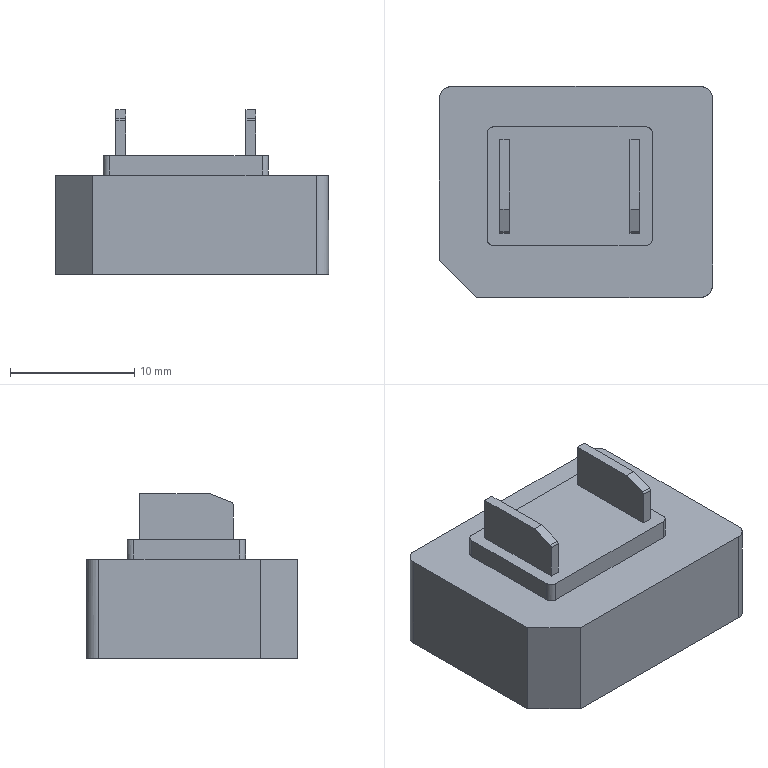NC program | PowerMill | posted by the shop | part box 22 x 17 x 13.286 mm
Lines 2696 to 5761 of 53717, first 2486 of 3066 lines:
( TOOL ID   D4C_1_1 )
( TOOL DIA. 4. TIP RAD 0 LENGTH 60.44 )
( Z = -5.38 )
T2 M6
T3
G91 G28 Z0
G0 G90 G54
M08
S18000 M3
X0 Y0 M8
G43 Z9.805 H2
X3.3 Y-4.574
Z.812
G1 Z-.388 F3600
X3.393 Y-4.374 F6000
X3.66 Y-3.797
X3.365 Y-3.66
X3.172 Y-3.54
X2.782 Y-3.172
X2.684 Y-3.041
X2.491 Y-2.684
X2.351 Y-2.196
X2.324 Y-1.708
Y.732
X.436 Y.731
G2 X-.364 Y-.069 I-.8 J0
G1 X-.636
G2 X-1.436 Y.731 I0 J.8
G1 Y1.674
G2 X-.636 Y2.473 I.8 J0
G1 X-.364
G2 X.436 Y1.674 I0 J-.8
G1 Y.731
X2.324 Y.732
Y4.148
X2.366 Y4.637
X2.534 Y5.125
X2.684 Y5.38
X2.873 Y5.613
X3.172 Y5.874
X3.585 Y6.101
X4.148 Y6.239
X5.125 Y6.249
X5.613 Y6.195
X5.907 Y6.101
X6.101 Y6.01
X6.589 Y5.645
X6.959 Y5.125
X7.077 Y4.829
X7.126 Y4.637
X7.168 Y4.148
Y-1.708
X7.142 Y-2.196
X7.077 Y-2.481
X7.002 Y-2.684
X6.707 Y-3.172
X6.589 Y-3.309
X6.127 Y-3.66
X5.613 Y-3.863
X5.125 Y-3.917
X4.148 Y-3.908
X3.66 Y-3.797
X3.393 Y-4.374
X-3.504 Y-4.099
X-3.657 Y-3.941
X-4.103 Y-3.479
X-4.148 Y-3.523
X-4.365 Y-3.66
X-4.637 Y-3.789
X-5.125 Y-3.905
X-6.101 Y-3.917
X-6.589 Y-3.869
X-7.077 Y-3.69
X-7.565 Y-3.333
X-7.709 Y-3.172
X-8.002 Y-2.684
X-8.142 Y-2.196
X-8.168 Y-1.708
Y4.148
X-8.126 Y4.637
X-8.053 Y4.901
X-7.959 Y5.125
X-7.62 Y5.613
X-7.077 Y6.023
X-6.908 Y6.101
X-6.589 Y6.2
X-6.101 Y6.249
X-5.125 Y6.237
X-4.637 Y6.121
X-4.148 Y5.857
X-3.873 Y5.613
X-3.66 Y5.345
X-3.534 Y5.125
X-3.366 Y4.637
X-3.324 Y4.148
Y-1.708
X-3.351 Y-2.196
X-3.49 Y-2.684
X-3.66 Y-3.005
X-3.786 Y-3.172
X-4.103 Y-3.479
X-3.657 Y-3.941
X2.918 Y-4.872 Z-.581
X3.035 Y-4.686
X3.373 Y-4.148
X3.172 Y-4.022
X2.789 Y-3.66
X2.684 Y-3.523
X2.493 Y-3.172
X2.351 Y-2.684
X2.324 Y-2.196
Y.972
X.436 Y.971
Y.268
G2 X-.367 Y-.532 I-.8 J0
G1 X-.639 Y-.531
G2 X-1.436 Y.269 I.003 J.8
G1 Y1.673
G2 X-.636 Y2.473 I.8 J0
G1 X-.364
G2 X.436 Y1.674 I0 J-.8
G1 Y.971
X2.324 Y.972
Y4.148
X2.366 Y4.637
X2.534 Y5.125
X2.684 Y5.38
X2.873 Y5.613
X3.172 Y5.874
X3.585 Y6.101
X4.148 Y6.239
X5.125 Y6.249
X5.613 Y6.195
X5.907 Y6.101
X6.101 Y6.01
X6.589 Y5.645
X6.959 Y5.125
X7.077 Y4.829
X7.127 Y4.637
X7.168 Y4.148
Y-2.196
X7.14 Y-2.684
X7.077 Y-2.963
X7. Y-3.172
X6.702 Y-3.66
X6.589 Y-3.791
X6.117 Y-4.148
X5.613 Y-4.345
X5.125 Y-4.4
X4.148 Y-4.39
X3.66 Y-4.28
X3.373 Y-4.148
X3.035 Y-4.686
G0 Z3.619
G1 X-8.196 Y-4.385 F10000
G0 Z.619
G1 Z-.581 F3600
X-8.033 Y-4.238 F6000
X-7.565 Y-3.815
X-7.704 Y-3.66
X-8. Y-3.172
X-8.141 Y-2.684
X-8.168 Y-2.196
Y4.148
X-8.126 Y4.637
X-8.053 Y4.901
X-7.959 Y5.125
X-7.62 Y5.613
X-7.077 Y6.023
X-6.908 Y6.101
X-6.589 Y6.2
X-6.101 Y6.249
X-5.125 Y6.237
X-4.637 Y6.121
X-4.148 Y5.857
X-3.873 Y5.613
X-3.66 Y5.345
X-3.534 Y5.125
X-3.366 Y4.637
X-3.324 Y4.148
Y-2.196
X-3.352 Y-2.684
X-3.493 Y-3.172
X-3.66 Y-3.487
X-3.79 Y-3.66
X-4.148 Y-4.005
X-4.374 Y-4.148
X-4.637 Y-4.271
X-5.125 Y-4.388
X-6.101 Y-4.4
X-6.589 Y-4.351
X-7.077 Y-4.172
X-7.565 Y-3.815
X-8.033 Y-4.238
G0 Z3.426
G1 X4.75 Y-5.738 F10000
G0 Z.426
G1 Z-.774 F3600
X4.752 Y-5.518 F6000
X4.759 Y-4.878
X4.148 Y-4.873
X3.66 Y-4.762
X3.385 Y-4.637
X3.172 Y-4.505
X2.795 Y-4.148
X2.684 Y-4.005
X2.496 Y-3.66
X2.352 Y-3.172
X2.324 Y-2.684
Y.725
X.436 Y.724
X.437 Y-.225
G2 X-.367 Y-1.025 I-.8 J0
G1 X-.639 Y-1.024
G2 X-1.436 Y-.224 I.004 J.8
G1 Y1.673
G2 X-.636 Y2.473 I.8 J0
G1 X-.364
G2 X.436 Y1.674 I0 J-.8
G1 Y.724
X2.324 Y.725
Y4.148
X2.366 Y4.637
X2.534 Y5.125
X2.684 Y5.38
X2.873 Y5.613
X3.172 Y5.874
X3.585 Y6.101
X4.148 Y6.239
X5.125 Y6.249
X5.613 Y6.195
X5.907 Y6.101
X6.101 Y6.01
X6.589 Y5.645
X6.959 Y5.125
X7.077 Y4.829
X7.127 Y4.637
X7.168 Y4.148
Y-2.684
X7.14 Y-3.172
X7.077 Y-3.445
X6.998 Y-3.66
X6.698 Y-4.148
X6.589 Y-4.273
X6.106 Y-4.637
X5.613 Y-4.828
X5.125 Y-4.882
X4.759 Y-4.878
X4.752 Y-5.518
X-2.974 Y-4.488
X-3.149 Y-4.355
X-3.66 Y-3.97
X-3.795 Y-4.148
X-4.148 Y-4.487
X-4.386 Y-4.637
X-4.637 Y-4.753
X-5.125 Y-4.87
X-6.101 Y-4.882
X-6.589 Y-4.833
X-7.077 Y-4.654
X-7.565 Y-4.297
X-7.698 Y-4.148
X-7.998 Y-3.66
X-8.14 Y-3.172
X-8.168 Y-2.684
Y4.148
X-8.126 Y4.637
X-8.053 Y4.901
X-7.959 Y5.125
X-7.62 Y5.613
X-7.077 Y6.023
X-6.908 Y6.101
X-6.589 Y6.2
X-6.101 Y6.249
X-5.125 Y6.237
X-4.637 Y6.121
X-4.148 Y5.857
X-3.873 Y5.613
X-3.66 Y5.345
X-3.534 Y5.125
X-3.366 Y4.637
X-3.324 Y4.148
Y-.092
Y-2.196
Y-2.198
Y-2.2
Y-2.684
X-3.352 Y-3.172
X-3.495 Y-3.66
X-3.66 Y-3.97
X-3.149 Y-4.355
G0 Z3.233
G1 X7.163 Y-5.334 F10000
G0 Z.233
G1 Z-.967 F3600
X7.029 Y-5.16 F6000
X6.624 Y-4.637
X6.101 Y-5.041
X5.922 Y-5.125
X5.613 Y-5.225
X5.125 Y-5.278
X4.148 Y-5.27
X3.66 Y-5.161
X3.172 Y-4.905
X2.868 Y-4.637
X2.684 Y-4.408
X2.532 Y-4.148
X2.368 Y-3.66
X2.324 Y-3.172
Y-2.689
Y-2.686
Y-2.684
Y.519
Y.529
X.429 Y.518
X.436 Y-.665
G2 X-.364 Y-1.47 I-.8 J-.005
G1 X-.636
G2 X-1.436 Y-.665 I0 J.8
G1 X-1.422 Y1.701
G2 X-.623 Y2.497 I.8 J-.005
G1 X-.378
G2 X.422 Y1.701 I0 J-.8
G1 X.429 Y.518
X2.324 Y.529
Y4.148
X2.366 Y4.637
X2.534 Y5.125
X2.684 Y5.38
X2.873 Y5.613
X3.172 Y5.874
X3.585 Y6.101
X4.148 Y6.239
X5.125 Y6.249
X5.613 Y6.195
X5.907 Y6.101
X6.101 Y6.01
X6.589 Y5.645
X6.959 Y5.125
X7.077 Y4.829
X7.127 Y4.637
X7.168 Y4.148
Y-3.172
X7.126 Y-3.66
X7.077 Y-3.854
X6.96 Y-4.148
X6.624 Y-4.637
X7.029 Y-5.16
G0 Z3.233
G1 X-5.116 Y-6.152 F10000
G0 Z.233
G1 Z-.967 F3600
X-5.118 Y-5.932 F6000
X-5.125 Y-5.269
X-6.101 Y-5.278
X-6.589 Y-5.232
X-7.077 Y-5.054
X-7.565 Y-4.698
X-7.959 Y-4.148
X-8.053 Y-3.926
X-8.124 Y-3.66
X-8.168 Y-3.172
Y4.148
X-8.127 Y4.637
X-8.053 Y4.901
X-7.959 Y5.125
X-7.62 Y5.613
X-7.077 Y6.023
X-6.908 Y6.101
X-6.589 Y6.2
X-6.101 Y6.249
X-5.125 Y6.237
X-4.637 Y6.121
X-4.148 Y5.857
X-3.873 Y5.613
X-3.66 Y5.345
X-3.534 Y5.125
X-3.366 Y4.637
X-3.324 Y4.148
Y-3.172
X-3.366 Y-3.66
X-3.533 Y-4.148
X-3.66 Y-4.372
X-3.869 Y-4.637
X-4.148 Y-4.887
X-4.569 Y-5.125
X-5.125 Y-5.269
X-5.118 Y-5.932
G0 Z3.04
G1 X2.135 Y6.114 F10000
G0 Z.04
G1 Z-1.16 F3600
X2.306 Y5.975 F6000
X2.825 Y5.554
X2.873 Y5.613
X3.172 Y5.874
X3.585 Y6.101
X4.148 Y6.239
X5.125 Y6.249
X5.613 Y6.195
X5.907 Y6.101
X6.101 Y6.01
X6.589 Y5.645
X6.959 Y5.125
X7.077 Y4.829
X7.127 Y4.637
X7.168 Y4.148
Y-3.172
X7.138 Y-3.66
X7.077 Y-3.915
X6.988 Y-4.148
X6.675 Y-4.637
X6.589 Y-4.731
X6.045 Y-5.125
X5.613 Y-5.28
X5.125 Y-5.334
X4.148 Y-5.325
X3.66 Y-5.215
X3.447 Y-5.125
X3.172 Y-4.96
X2.817 Y-4.637
X2.684 Y-4.466
X2.504 Y-4.148
X2.354 Y-3.66
X2.324 Y-3.172
Y.457
X.436
Y-.759
G2 X-.364 Y-1.559 I-.8 J0
G1 X-.636
G2 X-1.436 Y-.759 I0 J.8
G1 Y1.673
G2 X-.636 Y2.473 I.8 J0
G1 X-.364
G2 X.436 Y1.673 I0 J-.8
G1 Y.457
X2.324
Y4.148
X2.366 Y4.637
X2.534 Y5.125
X2.684 Y5.38
X2.825 Y5.554
X2.306 Y5.975
G0 Z3.04
G1 X-8.682 Y5.627 F10000
G0 Z.04
G1 Z-1.16 F3600
X-8.501 Y5.501 F6000
X-7.959 Y5.125
X-7.62 Y5.613
X-7.077 Y6.023
X-6.908 Y6.101
X-6.589 Y6.2
X-6.101 Y6.249
X-5.125 Y6.237
X-4.637 Y6.121
X-4.148 Y5.857
X-3.873 Y5.613
X-3.66 Y5.345
X-3.534 Y5.125
X-3.366 Y4.637
X-3.324 Y4.148
Y-3.172
X-3.354 Y-3.66
X-3.504 Y-4.148
X-3.66 Y-4.431
X-3.817 Y-4.637
X-4.148 Y-4.943
X-4.447 Y-5.125
X-4.637 Y-5.206
X-5.125 Y-5.322
X-6.101 Y-5.334
X-6.589 Y-5.286
X-7.045 Y-5.125
X-7.565 Y-4.754
X-7.675 Y-4.637
X-7.988 Y-4.148
X-8.138 Y-3.66
X-8.168 Y-3.172
Y4.148
X-8.127 Y4.637
X-8.053 Y4.901
X-7.959 Y5.125
X-8.501 Y5.501
G0 Z2.847
G1 X2.135 Y6.114 F10000
G0 Z-.153
G1 Z-1.353 F3600
X2.306 Y5.975 F6000
X2.825 Y5.554
X2.873 Y5.613
X3.172 Y5.874
X3.585 Y6.101
X4.148 Y6.239
X5.125 Y6.249
X5.613 Y6.195
X5.907 Y6.101
X6.101 Y6.01
X6.589 Y5.645
X6.959 Y5.125
X7.077 Y4.829
X7.127 Y4.637
X7.168 Y4.148
Y-3.172
X7.138 Y-3.66
X7.077 Y-3.915
X6.988 Y-4.148
X6.675 Y-4.637
X6.589 Y-4.731
X6.045 Y-5.125
X5.613 Y-5.28
X5.125 Y-5.334
X4.148 Y-5.325
X3.66 Y-5.215
X3.447 Y-5.125
X3.172 Y-4.96
X2.817 Y-4.637
X2.684 Y-4.466
X2.504 Y-4.148
X2.354 Y-3.66
X2.324 Y-3.172
Y.457
X.436
Y-.759
G2 X-.364 Y-1.559 I-.8 J0
G1 X-.636
G2 X-1.436 Y-.759 I0 J.8
G1 Y1.673
G2 X-.636 Y2.473 I.8 J0
G1 X-.364
G2 X.436 Y1.673 I0 J-.8
G1 Y.457
X2.324
Y4.148
X2.366 Y4.637
X2.534 Y5.125
X2.684 Y5.38
X2.825 Y5.554
X2.306 Y5.975
G0 Z2.847
G1 X-8.682 Y5.627 F10000
G0 Z-.153
G1 Z-1.353 F3600
X-8.501 Y5.501 F6000
X-7.959 Y5.125
X-7.62 Y5.613
X-7.077 Y6.023
X-6.908 Y6.101
X-6.589 Y6.2
X-6.101 Y6.249
X-5.125 Y6.237
X-4.637 Y6.121
X-4.148 Y5.857
X-3.873 Y5.613
X-3.66 Y5.345
X-3.534 Y5.125
X-3.366 Y4.637
X-3.324 Y4.148
Y-3.172
X-3.354 Y-3.66
X-3.504 Y-4.148
X-3.66 Y-4.431
X-3.817 Y-4.637
X-4.148 Y-4.943
X-4.447 Y-5.125
X-4.637 Y-5.206
X-5.125 Y-5.322
X-6.101 Y-5.334
X-6.589 Y-5.286
X-7.045 Y-5.125
X-7.565 Y-4.754
X-7.675 Y-4.637
X-7.988 Y-4.148
X-8.138 Y-3.66
X-8.168 Y-3.172
Y4.148
X-8.127 Y4.637
X-8.053 Y4.901
X-7.959 Y5.125
X-8.501 Y5.501
G0 Z2.813
G1 X2.135 Y6.114 F10000
G0 Z-.345
G1 Z-1.545 F3600
X2.306 Y5.975 F6000
X2.825 Y5.554
X2.873 Y5.613
X3.172 Y5.874
X3.585 Y6.101
X4.148 Y6.239
X5.125 Y6.249
X5.613 Y6.195
X5.907 Y6.101
X6.101 Y6.01
X6.589 Y5.645
X6.959 Y5.125
X7.077 Y4.829
X7.127 Y4.637
X7.168 Y4.148
Y-3.172
X7.138 Y-3.66
X7.077 Y-3.915
X6.988 Y-4.148
X6.675 Y-4.637
X6.589 Y-4.731
X6.045 Y-5.125
X5.613 Y-5.28
X5.125 Y-5.334
X4.148 Y-5.325
X3.66 Y-5.215
X3.447 Y-5.125
X3.172 Y-4.96
X2.817 Y-4.637
X2.684 Y-4.466
X2.504 Y-4.148
X2.354 Y-3.66
X2.324 Y-3.172
Y.457
X.436
Y-.759
G2 X-.364 Y-1.559 I-.8 J0
G1 X-.636
G2 X-1.436 Y-.759 I0 J.8
G1 Y1.673
G2 X-.636 Y2.473 I.8 J0
G1 X-.364
G2 X.436 Y1.673 I0 J-.8
G1 Y.457
X2.324
Y4.148
X2.366 Y4.637
X2.534 Y5.125
X2.684 Y5.38
X2.825 Y5.554
X2.306 Y5.975
G0 Z2.813
G1 X-8.682 Y5.627 F10000
G0 Z-.345
G1 Z-1.545 F3600
X-8.501 Y5.501 F6000
X-7.959 Y5.125
X-7.62 Y5.613
X-7.077 Y6.023
X-6.908 Y6.101
X-6.589 Y6.2
X-6.101 Y6.249
X-5.125 Y6.237
X-4.637 Y6.121
X-4.148 Y5.857
X-3.873 Y5.613
X-3.66 Y5.345
X-3.534 Y5.125
X-3.366 Y4.637
X-3.324 Y4.148
Y-3.172
X-3.354 Y-3.66
X-3.504 Y-4.148
X-3.66 Y-4.431
X-3.817 Y-4.637
X-4.148 Y-4.943
X-4.447 Y-5.125
X-4.637 Y-5.207
X-5.125 Y-5.323
X-6.101 Y-5.334
X-6.589 Y-5.286
X-7.045 Y-5.125
X-7.565 Y-4.754
X-7.675 Y-4.637
X-7.988 Y-4.148
X-8.138 Y-3.66
X-8.168 Y-3.172
Y4.148
X-8.127 Y4.637
X-8.053 Y4.901
X-7.959 Y5.125
X-8.501 Y5.501
G0 Z2.946
G1 X2.135 Y6.114 F10000
G0 Z-.538
G1 Z-1.738 F3600
X2.306 Y5.975 F6000
X2.825 Y5.554
X2.873 Y5.613
X3.172 Y5.874
X3.585 Y6.101
X4.148 Y6.239
X5.125 Y6.249
X5.613 Y6.195
X5.908 Y6.101
X6.101 Y6.01
X6.589 Y5.645
X6.959 Y5.125
X7.077 Y4.829
X7.127 Y4.637
X7.168 Y4.148
Y-3.172
X7.138 Y-3.66
X7.077 Y-3.915
X6.988 Y-4.148
X6.675 Y-4.637
X6.589 Y-4.731
X6.045 Y-5.125
X5.613 Y-5.28
X5.125 Y-5.334
X4.148 Y-5.325
X3.66 Y-5.215
X3.447 Y-5.125
X3.172 Y-4.96
X2.817 Y-4.637
X2.684 Y-4.466
X2.504 Y-4.148
X2.354 Y-3.66
X2.324 Y-3.172
Y.457
X.436
Y-.759
G2 X-.364 Y-1.559 I-.8 J0
G1 X-.636
G2 X-1.436 Y-.759 I0 J.8
G1 Y1.673
G2 X-.636 Y2.473 I.8 J0
G1 X-.364
G2 X.436 Y1.673 I0 J-.8
G1 Y.457
X2.324
Y4.148
X2.366 Y4.637
X2.534 Y5.125
X2.684 Y5.38
X2.825 Y5.554
X2.306 Y5.975
G0 Z2.946
G1 X-8.682 Y5.627 F10000
G0 Z-.538
G1 Z-1.738 F3600
X-8.501 Y5.501 F6000
X-7.959 Y5.125
X-7.62 Y5.613
X-7.077 Y6.023
X-6.908 Y6.101
X-6.589 Y6.2
X-6.101 Y6.249
X-5.125 Y6.237
X-4.637 Y6.121
X-4.148 Y5.857
X-3.873 Y5.613
X-3.66 Y5.345
X-3.534 Y5.125
X-3.366 Y4.637
X-3.324 Y4.148
Y-3.172
X-3.354 Y-3.66
X-3.504 Y-4.148
X-3.66 Y-4.431
X-3.817 Y-4.637
X-4.148 Y-4.943
X-4.447 Y-5.125
X-4.637 Y-5.207
X-5.125 Y-5.323
X-6.101 Y-5.334
X-6.589 Y-5.286
X-7.045 Y-5.125
X-7.565 Y-4.754
X-7.675 Y-4.637
X-7.988 Y-4.148
X-8.138 Y-3.66
X-8.168 Y-3.172
Y4.148
X-8.127 Y4.637
X-8.053 Y4.901
X-7.959 Y5.125
X-8.501 Y5.501
G0 Z2.927
G1 X6.629 Y6.717 F10000
G0 Z-.731
G1 Z-1.931 F3600
X6.498 Y6.54 F6000
X6.101 Y6.01
X6.589 Y5.645
X6.959 Y5.125
X7.077 Y4.829
X7.127 Y4.637
X7.168 Y4.148
Y-3.172
X7.138 Y-3.66
X7.077 Y-3.915
X6.988 Y-4.148
X6.675 Y-4.637
X6.589 Y-4.731
X6.045 Y-5.125
X5.613 Y-5.28
X5.125 Y-5.335
X4.148 Y-5.325
X3.66 Y-5.215
X3.447 Y-5.125
X3.172 Y-4.96
X2.817 Y-4.637
X2.684 Y-4.466
X2.504 Y-4.148
X2.354 Y-3.66
X2.324 Y-3.172
Y.457
X.436
Y-.759
G2 X-.364 Y-1.559 I-.8 J0
G1 X-.636
G2 X-1.436 Y-.759 I0 J.8
G1 Y1.673
G2 X-.636 Y2.473 I.8 J0
G1 X-.364
G2 X.436 Y1.673 I0 J-.8
G1 Y.457
X2.324
Y4.148
X2.366 Y4.637
X2.533 Y5.125
X2.684 Y5.38
X2.873 Y5.613
X3.172 Y5.874
X3.585 Y6.101
X4.148 Y6.239
X5.125 Y6.249
X5.613 Y6.195
X5.908 Y6.101
X6.101 Y6.01
X6.498 Y6.54
G0 Z2.927
G1 X-8.682 Y5.627 F10000
G0 Z-.731
G1 Z-1.931 F3600
X-8.501 Y5.501 F6000
X-7.959 Y5.125
X-7.62 Y5.613
X-7.077 Y6.023
X-6.908 Y6.101
X-6.589 Y6.2
X-6.101 Y6.249
X-5.125 Y6.237
X-4.637 Y6.121
X-4.148 Y5.857
X-3.873 Y5.613
X-3.66 Y5.345
X-3.534 Y5.125
X-3.366 Y4.637
X-3.324 Y4.148
Y-3.172
X-3.354 Y-3.66
X-3.504 Y-4.148
X-3.66 Y-4.431
X-3.817 Y-4.637
X-4.148 Y-4.943
X-4.447 Y-5.125
X-4.637 Y-5.207
X-5.125 Y-5.323
X-6.101 Y-5.335
X-6.589 Y-5.286
X-7.045 Y-5.125
X-7.565 Y-4.754
X-7.675 Y-4.637
X-7.988 Y-4.148
X-8.138 Y-3.66
X-8.168 Y-3.172
Y4.148
X-8.127 Y4.637
X-8.053 Y4.901
X-7.959 Y5.125
X-8.501 Y5.501
G0 Z2.914
G1 X6.629 Y6.717 F10000
G0 Z-.924
G1 Z-2.124 F3600
X6.498 Y6.54 F6000
X6.101 Y6.01
X6.589 Y5.645
X6.959 Y5.125
X7.077 Y4.829
X7.127 Y4.637
X7.168 Y4.148
Y-3.172
X7.138 Y-3.66
X7.077 Y-3.915
X6.988 Y-4.148
X6.676 Y-4.637
X6.589 Y-4.731
X6.045 Y-5.125
X5.613 Y-5.28
X5.125 Y-5.335
X4.148 Y-5.325
X3.66 Y-5.215
X3.447 Y-5.125
X3.172 Y-4.96
X2.817 Y-4.637
X2.684 Y-4.466
X2.504 Y-4.148
X2.354 Y-3.66
X2.324 Y-3.172
Y.457
X.436
Y-.759
G2 X-.364 Y-1.559 I-.8 J0
G1 X-.636
G2 X-1.436 Y-.759 I0 J.8
G1 Y1.673
G2 X-.636 Y2.473 I.8 J0
G1 X-.364
G2 X.436 Y1.673 I0 J-.8
G1 Y.457
X2.324
Y4.148
X2.366 Y4.637
X2.533 Y5.125
X2.684 Y5.38
X2.873 Y5.613
X3.172 Y5.874
X3.585 Y6.101
X4.148 Y6.239
X5.125 Y6.249
X5.613 Y6.195
X5.908 Y6.101
X6.101 Y6.01
X6.498 Y6.54
G0 Z2.914
G1 X-8.682 Y5.627 F10000
G0 Z-.924
G1 Z-2.124 F3600
X-8.501 Y5.501 F6000
X-7.959 Y5.125
X-7.62 Y5.613
X-7.077 Y6.023
X-6.908 Y6.101
X-6.589 Y6.2
X-6.101 Y6.249
X-5.125 Y6.237
X-4.637 Y6.121
X-4.148 Y5.857
X-3.873 Y5.613
X-3.66 Y5.345
X-3.534 Y5.125
X-3.366 Y4.637
X-3.324 Y4.148
Y-3.172
X-3.354 Y-3.66
X-3.504 Y-4.148
X-3.66 Y-4.431
X-3.817 Y-4.637
X-4.148 Y-4.943
X-4.447 Y-5.125
X-4.637 Y-5.207
X-5.125 Y-5.323
X-6.101 Y-5.335
X-6.589 Y-5.286
X-7.045 Y-5.125
X-7.565 Y-4.754
X-7.675 Y-4.637
X-7.988 Y-4.148
X-8.138 Y-3.66
X-8.168 Y-3.172
Y4.148
X-8.127 Y4.637
X-8.053 Y4.901
X-7.959 Y5.125
X-8.501 Y5.501
G0 Z2.907
G1 X6.629 Y6.717 F10000
G0 Z-1.117
G1 Z-2.317 F3600
X6.498 Y6.54 F6000
X6.101 Y6.01
X6.589 Y5.645
X6.959 Y5.125
X7.077 Y4.829
X7.127 Y4.637
X7.168 Y4.148
Y-3.172
X7.138 Y-3.66
X7.077 Y-3.915
X6.988 Y-4.148
X6.676 Y-4.637
X6.589 Y-4.731
X6.045 Y-5.125
X5.613 Y-5.28
X5.125 Y-5.335
X4.148 Y-5.325
X3.66 Y-5.215
X3.447 Y-5.125
X3.172 Y-4.96
X2.817 Y-4.637
X2.684 Y-4.466
X2.504 Y-4.148
X2.354 Y-3.66
X2.324 Y-3.172
Y.457
X.436
Y-.759
G2 X-.364 Y-1.559 I-.8 J0
G1 X-.636
G2 X-1.436 Y-.759 I0 J.8
G1 Y1.673
G2 X-.636 Y2.473 I.8 J0
G1 X-.364
G2 X.436 Y1.673 I0 J-.8
G1 Y.457
X2.324
Y4.148
X2.366 Y4.637
X2.533 Y5.125
X2.684 Y5.38
X2.873 Y5.613
X3.172 Y5.874
X3.585 Y6.101
X4.148 Y6.239
X5.125 Y6.249
X5.613 Y6.195
X5.908 Y6.101
X6.101 Y6.01
X6.498 Y6.54
G0 Z2.907
G1 X-8.682 Y5.627 F10000
G0 Z-1.117
G1 Z-2.317 F3600
X-8.501 Y5.501 F6000
X-7.959 Y5.125
X-7.62 Y5.613
X-7.077 Y6.023
X-6.908 Y6.101
X-6.589 Y6.2
X-6.101 Y6.249
X-5.125 Y6.237
X-4.637 Y6.121
X-4.148 Y5.857
X-3.873 Y5.613
X-3.66 Y5.345
X-3.534 Y5.125
X-3.366 Y4.637
X-3.324 Y4.148
Y-3.172
X-3.354 Y-3.66
X-3.504 Y-4.148
X-3.66 Y-4.431
X-3.817 Y-4.637
X-4.148 Y-4.943
X-4.447 Y-5.125
X-4.637 Y-5.207
X-5.125 Y-5.323
X-6.101 Y-5.335
X-6.589 Y-5.286
X-7.045 Y-5.125
X-7.565 Y-4.754
X-7.675 Y-4.637
X-7.988 Y-4.148
X-8.138 Y-3.66
X-8.168 Y-3.172
Y4.148
X-8.127 Y4.637
X-8.053 Y4.901
X-7.959 Y5.125
X-8.501 Y5.501
G0 Z2.906
G1 X6.629 Y6.717 F10000
G0 Z-1.31
G1 Z-2.51 F3600
X6.498 Y6.54 F6000
X6.101 Y6.01
X6.589 Y5.645
X6.959 Y5.125
X7.077 Y4.829
X7.127 Y4.637
X7.168 Y4.148
Y-3.172
X7.138 Y-3.66
X7.077 Y-3.915
X6.988 Y-4.148
X6.676 Y-4.637
X6.589 Y-4.731
X6.045 Y-5.125
X5.613 Y-5.28
X5.125 Y-5.335
X4.148 Y-5.325
X3.66 Y-5.215
X3.447 Y-5.125
X3.172 Y-4.96
X2.817 Y-4.637
X2.684 Y-4.466
X2.504 Y-4.148
X2.354 Y-3.66
X2.324 Y-3.172
Y.457
X.436
Y-.759
G2 X-.364 Y-1.559 I-.8 J0
G1 X-.636
G2 X-1.436 Y-.759 I0 J.8
G1 Y1.673
G2 X-.636 Y2.473 I.8 J0
G1 X-.364
G2 X.436 Y1.674 I0 J-.8
G1 Y.457
X2.324
Y4.148
X2.366 Y4.637
X2.533 Y5.125
X2.684 Y5.38
X2.873 Y5.613
X3.172 Y5.874
X3.585 Y6.101
X4.148 Y6.239
X5.125 Y6.249
X5.613 Y6.195
X5.908 Y6.101
X6.101 Y6.01
X6.498 Y6.54
G0 Z2.906
G1 X-8.682 Y5.627 F10000
G0 Z-1.31
G1 Z-2.51 F3600
X-8.501 Y5.501 F6000
X-7.959 Y5.125
X-7.62 Y5.613
X-7.077 Y6.023
X-6.908 Y6.101
X-6.589 Y6.2
X-6.101 Y6.249
X-5.125 Y6.237
X-4.637 Y6.121
X-4.148 Y5.857
X-3.872 Y5.613
X-3.66 Y5.345
X-3.534 Y5.125
X-3.366 Y4.637
X-3.324 Y4.148
Y-3.172
X-3.354 Y-3.66
X-3.504 Y-4.148
X-3.66 Y-4.431
X-3.817 Y-4.637
X-4.148 Y-4.943
X-4.447 Y-5.125
X-4.637 Y-5.207
X-5.125 Y-5.323
X-6.101 Y-5.335
X-6.589 Y-5.286
X-7.045 Y-5.125
X-7.565 Y-4.754
X-7.676 Y-4.637
X-7.988 Y-4.148
X-8.138 Y-3.66
X-8.168 Y-3.172
Y4.148
X-8.127 Y4.637
X-8.053 Y4.901
X-7.959 Y5.125
X-8.501 Y5.501
G0 Z2.911
G1 X6.629 Y6.717 F10000
G0 Z-1.503
G1 Z-2.703 F3600
X6.498 Y6.54 F6000
X6.101 Y6.01
X6.589 Y5.645
X6.959 Y5.125
X7.077 Y4.829
X7.127 Y4.637
X7.168 Y4.148
Y-3.172
X7.138 Y-3.66
X7.077 Y-3.915
X6.988 Y-4.148
X6.676 Y-4.637
X6.589 Y-4.731
X6.045 Y-5.125
X5.613 Y-5.28
X5.125 Y-5.335
X4.148 Y-5.325
X3.66 Y-5.215
X3.447 Y-5.125
X3.172 Y-4.96
X2.817 Y-4.637
X2.684 Y-4.466
X2.504 Y-4.148
X2.354 Y-3.66
X2.324 Y-3.172
Y.457
X.436
Y-.759
G2 X-.364 Y-1.559 I-.8 J0
G1 X-.636
G2 X-1.436 Y-.759 I0 J.8
G1 Y1.674
G2 X-.636 Y2.473 I.8 J0
G1 X-.364 Y2.474
G2 X.436 Y1.674 I0 J-.8
G1 Y.457
X2.324
Y4.148
X2.366 Y4.637
X2.533 Y5.125
X2.684 Y5.38
X2.873 Y5.613
X3.172 Y5.874
X3.585 Y6.101
X4.148 Y6.239
X5.125 Y6.249
X5.613 Y6.195
X5.908 Y6.101
X6.101 Y6.01
X6.498 Y6.54
G0 Z2.911
G1 X-8.682 Y5.627 F10000
G0 Z-1.503
G1 Z-2.703 F3600
X-8.501 Y5.501 F6000
X-7.959 Y5.125
X-7.62 Y5.613
X-7.077 Y6.023
X-6.908 Y6.101
X-6.589 Y6.2
X-6.101 Y6.249
X-5.125 Y6.237
X-4.637 Y6.121
X-4.148 Y5.857
X-3.872 Y5.613
X-3.66 Y5.345
X-3.534 Y5.125
X-3.366 Y4.637
X-3.324 Y4.148
Y-3.172
X-3.354 Y-3.66
X-3.504 Y-4.148
X-3.66 Y-4.431
X-3.817 Y-4.637
X-4.148 Y-4.943
X-4.447 Y-5.125
X-4.637 Y-5.207
X-5.125 Y-5.323
X-6.101 Y-5.335
X-6.589 Y-5.286
X-7.045 Y-5.125
X-7.565 Y-4.754
X-7.676 Y-4.637
X-7.988 Y-4.148
X-8.138 Y-3.66
X-8.168 Y-3.172
Y4.148
X-8.127 Y4.637
X-8.053 Y4.901
X-7.959 Y5.125
X-8.501 Y5.501
G0 Z2.921
G1 X6.629 Y6.717 F10000
G0 Z-1.696
G1 Z-2.896 F3600
X6.498 Y6.54 F6000
X6.101 Y6.01
X6.589 Y5.645
X6.959 Y5.125
X7.077 Y4.829
X7.127 Y4.637
X7.168 Y4.148
Y-3.172
X7.138 Y-3.66
X7.077 Y-3.915
X6.988 Y-4.148
X6.676 Y-4.637
X6.589 Y-4.731
X6.045 Y-5.125
X5.613 Y-5.28
X5.125 Y-5.335
X4.148 Y-5.325
X3.66 Y-5.215
X3.447 Y-5.125
X3.172 Y-4.96
X2.817 Y-4.637
X2.684 Y-4.466
X2.504 Y-4.148
X2.354 Y-3.66
X2.324 Y-3.172
Y.457
X.436
Y-.759
G2 X-.364 Y-1.559 I-.8 J0
G1 X-.636
G2 X-1.436 Y-.759 I0 J.8
G1 Y1.674
G2 X-.636 Y2.474 I.8 J0
G1 X-.364
G2 X.436 Y1.674 I0 J-.8
G1 Y.457
X2.324
Y4.148
X2.366 Y4.637
X2.533 Y5.125
X2.684 Y5.38
X2.872 Y5.613
X3.172 Y5.874
X3.585 Y6.101
X4.148 Y6.239
X5.125 Y6.249
X5.613 Y6.195
X5.908 Y6.101
X6.101 Y6.01
X6.498 Y6.54
G0 Z2.921
G1 X-8.682 Y5.627 F10000
G0 Z-1.696
G1 Z-2.896 F3600
X-8.501 Y5.501 F6000
X-7.959 Y5.125
X-7.62 Y5.613
X-7.077 Y6.023
X-6.908 Y6.101
X-6.589 Y6.2
X-6.101 Y6.249
X-5.125 Y6.237
X-4.637 Y6.121
X-4.148 Y5.857
X-3.872 Y5.613
X-3.66 Y5.345
X-3.533 Y5.125
X-3.366 Y4.637
X-3.324 Y4.148
Y-3.172
X-3.354 Y-3.66
X-3.504 Y-4.148
X-3.66 Y-4.431
X-3.817 Y-4.637
X-4.148 Y-4.943
X-4.447 Y-5.125
X-4.637 Y-5.207
X-5.125 Y-5.323
X-6.101 Y-5.335
X-6.589 Y-5.286
X-7.045 Y-5.125
X-7.565 Y-4.754
X-7.676 Y-4.637
X-7.988 Y-4.148
X-8.138 Y-3.66
X-8.168 Y-3.172
Y4.148
X-8.127 Y4.637
X-8.053 Y4.901
X-7.959 Y5.125
X-8.501 Y5.501
G0 Z2.938
G1 X6.629 Y6.717 F10000
G0 Z-1.889
G1 Z-3.089 F3600
X6.498 Y6.54 F6000
X6.101 Y6.01
X6.589 Y5.645
X6.959 Y5.125
X7.077 Y4.829
X7.127 Y4.637
X7.168 Y4.148
Y-3.172
X7.138 Y-3.66
X7.077 Y-3.915
X6.988 Y-4.148
X6.676 Y-4.637
X6.589 Y-4.731
X6.045 Y-5.125
X5.613 Y-5.28
X5.125 Y-5.335
X4.148 Y-5.325
X3.66 Y-5.215
X3.447 Y-5.125
X3.172 Y-4.96
X2.817 Y-4.637
X2.684 Y-4.466
X2.504 Y-4.148
X2.354 Y-3.66
X2.324 Y-3.172
Y.457
X.436
Y-.759
G2 X-.364 Y-1.559 I-.8 J0
G1 X-.636
G2 X-1.436 Y-.759 I0 J.8
G1 Y1.674
G2 X-.636 Y2.474 I.8 J0
G1 X-.364
G2 X.436 Y1.674 I0 J-.8
G1 Y.457
X2.324
Y4.148
X2.366 Y4.637
X2.533 Y5.125
X2.684 Y5.38
X2.872 Y5.613
X3.172 Y5.874
X3.585 Y6.101
X4.148 Y6.239
X5.125 Y6.249
X5.613 Y6.195
X5.908 Y6.101
X6.101 Y6.01
X6.498 Y6.54
G0 Z2.938
G1 X-8.682 Y5.627 F10000
G0 Z-1.889
G1 Z-3.089 F3600
X-8.501 Y5.501 F6000
X-7.959 Y5.125
X-7.62 Y5.613
X-7.077 Y6.023
X-6.908 Y6.101
X-6.589 Y6.2
X-6.101 Y6.249
X-5.125 Y6.237
X-4.637 Y6.121
X-4.148 Y5.857
X-3.872 Y5.613
X-3.66 Y5.345
X-3.533 Y5.125
X-3.366 Y4.637
X-3.324 Y4.148
Y-3.172
X-3.354 Y-3.66
X-3.504 Y-4.148
X-3.66 Y-4.431
X-3.817 Y-4.637
X-4.148 Y-4.943
X-4.447 Y-5.125
X-4.637 Y-5.207
X-5.125 Y-5.323
X-6.101 Y-5.335
X-6.589 Y-5.286
X-7.045 Y-5.125
X-7.565 Y-4.754
X-7.676 Y-4.637
X-7.988 Y-4.148
X-8.138 Y-3.66
X-8.168 Y-3.172
Y4.148
X-8.127 Y4.637
X-8.053 Y4.901
X-7.959 Y5.125
X-8.501 Y5.501
G0 Z2.961
G1 X6.629 Y6.717 F10000
G0 Z-2.082
G1 Z-3.282 F3600
X6.498 Y6.54 F6000
X6.101 Y6.01
X6.589 Y5.645
X6.959 Y5.125
X7.077 Y4.829
X7.127 Y4.637
X7.168 Y4.148
Y-3.172
X7.138 Y-3.66
X7.077 Y-3.915
X6.988 Y-4.148
X6.676 Y-4.637
X6.589 Y-4.731
X6.045 Y-5.125
X5.613 Y-5.28
X5.125 Y-5.335
X4.148 Y-5.325
X3.66 Y-5.215
X3.447 Y-5.125
X3.172 Y-4.96
X2.817 Y-4.637
X2.684 Y-4.466
X2.504 Y-4.148
X2.354 Y-3.66
X2.324 Y-3.172
Y.457
X.436
Y-.759
G2 X-.364 Y-1.559 I-.8 J0
G1 X-.636
G2 X-1.436 Y-.759 I0 J.8
G1 Y1.674
G2 X-.636 Y2.474 I.8 J0
G1 X-.364
G2 X.436 Y1.674 I0 J-.8
G1 Y.457
X2.324
Y4.148
X2.366 Y4.637
X2.533 Y5.125
X2.684 Y5.38
X2.872 Y5.613
X3.172 Y5.874
X3.585 Y6.101
X4.148 Y6.239
X5.125 Y6.249
X5.613 Y6.195
X5.908 Y6.101
X6.101 Y6.01
X6.498 Y6.54
G0 Z2.961
G1 X-8.682 Y5.627 F10000
G0 Z-2.082
G1 Z-3.282 F3600
X-8.501 Y5.501 F6000
X-7.959 Y5.125
X-7.62 Y5.613
X-7.077 Y6.023
X-6.908 Y6.101
X-6.589 Y6.2
X-6.101 Y6.249
X-5.125 Y6.237
X-4.637 Y6.121
X-4.148 Y5.857
X-3.872 Y5.613
X-3.66 Y5.345
X-3.533 Y5.125
X-3.366 Y4.637
X-3.324 Y4.148
Y-3.172
X-3.354 Y-3.66
X-3.504 Y-4.148
X-3.66 Y-4.431
X-3.817 Y-4.637
X-4.148 Y-4.943
X-4.447 Y-5.125
X-4.637 Y-5.207
X-5.125 Y-5.323
X-6.101 Y-5.335
X-6.589 Y-5.286
X-7.045 Y-5.125
X-7.565 Y-4.754
X-7.676 Y-4.637
X-7.988 Y-4.148
X-8.138 Y-3.66
X-8.168 Y-3.172
Y4.148
X-8.127 Y4.637
X-8.053 Y4.901
X-7.959 Y5.125
X-8.501 Y5.501
G0 Z2.99
G1 X6.629 Y6.717 F10000
G0 Z-2.275
G1 Z-3.475 F3600
X6.498 Y6.54 F6000
X6.101 Y6.01
X6.589 Y5.645
X6.959 Y5.125
X7.077 Y4.83
X7.127 Y4.637
X7.168 Y4.148
Y-3.172
X7.138 Y-3.66
X7.077 Y-3.915
X6.988 Y-4.148
X6.676 Y-4.637
X6.589 Y-4.731
X6.045 Y-5.125
X5.613 Y-5.28
X5.125 Y-5.335
X4.148 Y-5.325
X3.66 Y-5.215
X3.447 Y-5.125
X3.172 Y-4.96
X2.817 Y-4.637
X2.684 Y-4.466
X2.504 Y-4.148
X2.354 Y-3.66
X2.324 Y-3.172
Y.457
X.436
Y-.759
G2 X-.364 Y-1.559 I-.8 J0
G1 X-.636
G2 X-1.436 Y-.759 I0 J.8
G1 Y1.674
G2 X-.636 Y2.474 I.8 J0
G1 X-.364
G2 X.436 Y1.674 I0 J-.8
G1 Y.457
X2.324
Y4.148
X2.366 Y4.637
X2.533 Y5.125
X2.684 Y5.38
X2.872 Y5.613
X3.172 Y5.874
X3.585 Y6.101
X4.148 Y6.239
X5.125 Y6.249
X5.613 Y6.195
X5.908 Y6.101
X6.101 Y6.01
X6.498 Y6.54
G0 Z2.99
G1 X-8.682 Y5.627 F10000
G0 Z-2.275
G1 Z-3.475 F3600
X-8.501 Y5.501 F6000
X-7.959 Y5.125
X-7.62 Y5.613
X-7.077 Y6.023
X-6.908 Y6.101
X-6.589 Y6.2
X-6.101 Y6.249
X-5.125 Y6.237
X-4.637 Y6.121
X-4.148 Y5.857
X-3.872 Y5.613
X-3.66 Y5.345
X-3.533 Y5.125
X-3.366 Y4.637
X-3.324 Y4.148
Y-3.172
X-3.354 Y-3.66
X-3.504 Y-4.148
X-3.66 Y-4.431
X-3.817 Y-4.637
X-4.148 Y-4.943
X-4.447 Y-5.125
X-4.637 Y-5.207
X-5.125 Y-5.323
X-6.101 Y-5.335
X-6.589 Y-5.286
X-7.045 Y-5.125
X-7.565 Y-4.754
X-7.676 Y-4.637
X-7.988 Y-4.148
X-8.138 Y-3.66
X-8.168 Y-3.172
Y4.148
X-8.127 Y4.637
X-8.053 Y4.901
X-7.959 Y5.125
X-8.501 Y5.501
G0 Z2.834
G1 X6.629 Y6.717 F10000
G0 Z-2.468
G1 Z-3.668 F3600
X6.498 Y6.54 F6000
X6.101 Y6.01
X6.589 Y5.645
X6.959 Y5.125
X7.077 Y4.83
X7.127 Y4.637
X7.168 Y4.148
Y-3.172
X7.138 Y-3.66
X7.077 Y-3.915
X6.988 Y-4.148
X6.676 Y-4.637
X6.589 Y-4.731
X6.045 Y-5.125
X5.613 Y-5.28
X5.125 Y-5.335
X4.148 Y-5.325
X3.66 Y-5.215
X3.447 Y-5.125
X3.172 Y-4.96
X2.817 Y-4.637
X2.684 Y-4.466
X2.504 Y-4.148
X2.354 Y-3.66
X2.324 Y-3.172
Y.457
X.436
Y-.759
G2 X-.364 Y-1.559 I-.8 J0
G1 X-.636
G2 X-1.436 Y-.759 I0 J.8
G1 Y1.674
G2 X-.636 Y2.474 I.8 J0
G1 X-.364
G2 X.436 Y1.674 I0 J-.8
G1 Y.457
X2.324
Y4.148
X2.366 Y4.637
X2.533 Y5.125
X2.684 Y5.38
X2.872 Y5.613
X3.172 Y5.874
X3.585 Y6.101
X4.148 Y6.239
X5.125 Y6.249
X5.613 Y6.195
X5.908 Y6.101
X6.101 Y6.01
X6.498 Y6.54
G0 Z2.834
G1 X-8.682 Y5.627 F10000
G0 Z-2.468
G1 Z-3.668 F3600
X-8.501 Y5.501 F6000
X-7.959 Y5.125
X-7.62 Y5.613
X-7.077 Y6.023
X-6.908 Y6.101
X-6.589 Y6.2
X-6.101 Y6.249
X-5.125 Y6.237
X-4.637 Y6.121
X-4.148 Y5.857
X-3.872 Y5.613
X-3.66 Y5.345
X-3.533 Y5.125
X-3.366 Y4.637
X-3.324 Y4.148
Y-3.172
X-3.354 Y-3.66
X-3.504 Y-4.148
X-3.66 Y-4.431
X-3.817 Y-4.637
X-4.148 Y-4.943
X-4.447 Y-5.125
X-4.637 Y-5.207
X-5.125 Y-5.323
X-6.101 Y-5.335
X-6.589 Y-5.286
X-7.045 Y-5.125
X-7.565 Y-4.755
X-7.676 Y-4.637
X-7.988 Y-4.148
X-8.138 Y-3.66
X-8.168 Y-3.172
Y4.148
X-8.127 Y4.637
X-8.053 Y4.901
X-7.959 Y5.125
X-8.501 Y5.501
G0 Z2.872
G1 X6.653 Y6.749 F10000
G0 Z-2.661
G1 Z-3.861 F3600
X6.522 Y6.573 F6000
X6.101 Y6.01
X6.589 Y5.645
X6.959 Y5.125
X7.077 Y4.83
X7.127 Y4.637
X7.168 Y4.148
Y-3.172
X7.138 Y-3.66
X7.077 Y-3.915
X6.988 Y-4.148
X6.676 Y-4.637
X6.589 Y-4.731
X6.045 Y-5.125
X5.613 Y-5.28
X5.125 Y-5.335
X4.148 Y-5.325
X3.66 Y-5.215
X3.447 Y-5.125
X3.172 Y-4.96
X2.817 Y-4.637
X2.684 Y-4.466
X2.504 Y-4.148
X2.354 Y-3.66
X2.324 Y-3.172
Y.457
X.436
Y-.799
G2 X-.364 Y-1.599 I-.8 J0
G1 X-.636
G2 X-1.436 Y-.799 I0 J.8
G1 Y1.714
G2 X-.636 Y2.514 I.8 J0
G1 X-.364
G2 X.436 Y1.714 I0 J-.8
G1 Y.457
X2.324
Y4.148
X2.366 Y4.637
X2.533 Y5.125
X2.684 Y5.38
X2.872 Y5.613
X3.172 Y5.874
X3.585 Y6.101
X4.148 Y6.239
X5.125 Y6.249
X5.613 Y6.195
X5.908 Y6.101
X6.101 Y6.01
X6.522 Y6.573
G0 Z2.872
G1 X-8.715 Y5.65 F10000
G0 Z-2.661
G1 Z-3.861 F3600
X-8.534 Y5.524 F6000
X-7.959 Y5.125
X-7.62 Y5.613
X-7.077 Y6.023
X-6.908 Y6.101
X-6.589 Y6.2
X-6.101 Y6.249
X-5.125 Y6.237
X-4.637 Y6.121
X-4.148 Y5.857
X-3.872 Y5.613
X-3.66 Y5.345
X-3.533 Y5.125
X-3.366 Y4.637
X-3.324 Y4.148
Y-3.172
X-3.354 Y-3.66
X-3.504 Y-4.148
X-3.66 Y-4.431
X-3.817 Y-4.637
X-4.148 Y-4.943
X-4.447 Y-5.125
X-4.637 Y-5.207
X-5.125 Y-5.323
X-6.101 Y-5.335
X-6.589 Y-5.286
X-7.045 Y-5.125
X-7.565 Y-4.755
X-7.676 Y-4.637
X-7.988 Y-4.148
X-8.138 Y-3.66
X-8.168 Y-3.172
Y4.148
X-8.127 Y4.637
X-8.053 Y4.901
X-7.959 Y5.125
X-8.534 Y5.524
G0 Z2.918
G1 X-10.108 Y5.114 F10000
G0 Z-2.85
G1 Z-4.05 F3600
X-10.095 Y5.096 F6000
G3 X-9.817 Y5.059 I.157 J.12
G1 X-8.945 Y5.725
X-8.761 Y6.101
X-8.541 Y6.39
X-8.348 Y6.589
X-8.053 Y6.821
X-7.565 Y7.076
X-7.077 Y7.207
X-6.589 Y7.249
X5.613
X6.101 Y7.203
X6.563 Y7.077
X7.077 Y6.805
X7.348 Y6.589
X7.565 Y6.362
X7.761 Y6.101
X8.008 Y5.613
X8.131 Y5.125
X8.168 Y4.637
Y-3.66
X8.141 Y-4.148
X8.053 Y-4.568
X7.799 Y-5.125
X7.565 Y-5.447
X7.414 Y-5.613
X7.077 Y-5.89
X6.707 Y-6.101
X6.101 Y-6.289
X5.613 Y-6.335
X-6.589
X-7.077 Y-6.293
X-7.565 Y-6.162
X-8.053 Y-5.906
X-8.414 Y-5.613
X-8.541 Y-5.476
X-8.799 Y-5.125
X-9.029 Y-4.639
X-9.141 Y-4.148
X-9.168 Y-3.66
Y4.637
X-9.131 Y5.125
X-9.029 Y5.553
X-8.945 Y5.725
X-10.108 Y5.114 Z-4.24
X-10.095 Y5.096
G3 X-9.817 Y5.059 I.157 J.12
G1 X-8.945 Y5.725
X-8.761 Y6.101
X-8.541 Y6.39
X-8.348 Y6.589
X-8.053 Y6.821
X-7.565 Y7.076
X-7.077 Y7.207
X-6.589 Y7.249
X5.613
X6.101 Y7.203
X6.563 Y7.077
X7.077 Y6.805
X7.348 Y6.589
X7.565 Y6.362
X7.761 Y6.101
X8.008 Y5.613
X8.131 Y5.125
X8.168 Y4.637
Y-3.66
X8.141 Y-4.148
X8.053 Y-4.568
X7.799 Y-5.125
X7.565 Y-5.447
X7.414 Y-5.613
X7.077 Y-5.89
X6.707 Y-6.101
X6.101 Y-6.289
X5.613 Y-6.335
X-6.589
X-7.077 Y-6.293
X-7.565 Y-6.162
X-8.053 Y-5.906
X-8.414 Y-5.613
X-8.541 Y-5.476
X-8.799 Y-5.125
X-9.029 Y-4.639
X-9.141 Y-4.148
X-9.168 Y-3.66
Y4.637
X-9.131 Y5.125
X-9.029 Y5.553
X-8.945 Y5.725
X-10.108 Y5.114 Z-4.43
X-10.095 Y5.096
G3 X-9.817 Y5.059 I.157 J.12
G1 X-8.945 Y5.725
X-8.761 Y6.101
X-8.541 Y6.391
X-8.348 Y6.589
X-8.053 Y6.821
X-7.565 Y7.076
X-7.077 Y7.207
X-6.589 Y7.249
X5.613
X6.101 Y7.204
X6.563 Y7.077
X7.077 Y6.805
X7.348 Y6.589
X7.565 Y6.362
X7.761 Y6.101
X8.008 Y5.613
X8.131 Y5.125
X8.168 Y4.637
Y-3.66
X8.141 Y-4.148
X8.053 Y-4.568
X7.799 Y-5.125
X7.565 Y-5.447
X7.414 Y-5.613
X7.077 Y-5.89
X6.707 Y-6.101
X6.101 Y-6.289
X5.613 Y-6.335
X-6.589
X-7.077 Y-6.293
X-7.565 Y-6.162
X-8.053 Y-5.906
X-8.414 Y-5.613
X-8.541 Y-5.476
X-8.799 Y-5.125
X-9.029 Y-4.639
X-9.141 Y-4.148
X-9.168 Y-3.66
Y4.637
X-9.131 Y5.125
X-9.029 Y5.553
X-8.945 Y5.725
X-10.108 Y5.114 Z-4.62
X-10.095 Y5.096
G3 X-9.817 Y5.059 I.157 J.12
G1 X-8.945 Y5.725
X-8.761 Y6.101
X-8.541 Y6.391
X-8.348 Y6.589
X-8.053 Y6.821
X-7.565 Y7.076
X-7.077 Y7.207
X-6.589 Y7.249
X5.613
X6.101 Y7.204
X6.563 Y7.077
X7.077 Y6.805
X7.348 Y6.589
X7.565 Y6.362
X7.761 Y6.101
X8.008 Y5.613
X8.131 Y5.125
X8.168 Y4.637
Y-3.66
X8.141 Y-4.148
X8.053 Y-4.568
X7.799 Y-5.125
X7.565 Y-5.448
X7.414 Y-5.613
X7.077 Y-5.89
X6.707 Y-6.101
X6.101 Y-6.289
X5.613 Y-6.335
X-6.589
X-7.077 Y-6.293
X-7.565 Y-6.162
X-8.053 Y-5.906
X-8.414 Y-5.613
X-8.541 Y-5.476
X-8.799 Y-5.125
X-9.029 Y-4.639
X-9.141 Y-4.148
X-9.168 Y-3.66
Y4.637
X-9.131 Y5.125
X-9.029 Y5.553
X-8.945 Y5.725
X-10.108 Y5.114 Z-4.81
X-10.095 Y5.096
G3 X-9.817 Y5.059 I.157 J.12
G1 X-8.945 Y5.725
X-8.761 Y6.101
X-8.541 Y6.391
X-8.348 Y6.589
X-8.053 Y6.821
X-7.565 Y7.076
X-7.077 Y7.207
X-6.589 Y7.249
X5.613
X6.101 Y7.204
X6.563 Y7.077
X7.077 Y6.805
X7.348 Y6.589
X7.565 Y6.362
X7.761 Y6.101
X8.008 Y5.613
X8.131 Y5.125
X8.168 Y4.637
Y-3.66
X8.141 Y-4.148
X8.053 Y-4.568
X7.799 Y-5.125
X7.565 Y-5.448
X7.414 Y-5.613
X7.077 Y-5.89
X6.707 Y-6.101
X6.101 Y-6.289
X5.613 Y-6.335
X-6.589
X-7.077 Y-6.293
X-7.565 Y-6.162
X-8.053 Y-5.906
X-8.414 Y-5.613
X-8.541 Y-5.476
X-8.799 Y-5.125
X-9.029 Y-4.639
X-9.141 Y-4.148
X-9.168 Y-3.66
Y4.637
X-9.131 Y5.125
X-9.029 Y5.553
X-8.945 Y5.725
X-10.108 Y5.114 Z-5.
X-10.095 Y5.096
G3 X-9.817 Y5.059 I.157 J.12
G1 X-8.945 Y5.725
X-8.761 Y6.101
X-8.541 Y6.391
X-8.348 Y6.589
X-8.053 Y6.821
X-7.565 Y7.076
X-7.077 Y7.207
X-6.589 Y7.249
X5.613
X6.101 Y7.204
X6.563 Y7.077
X7.077 Y6.805
X7.348 Y6.589
X7.565 Y6.362
X7.761 Y6.101
X8.008 Y5.613
X8.131 Y5.125
X8.168 Y4.637
Y-3.66
X8.141 Y-4.148
X8.053 Y-4.568
X7.799 Y-5.125
X7.565 Y-5.448
X7.414 Y-5.613
X7.077 Y-5.89
X6.707 Y-6.101
X6.101 Y-6.289
X5.613 Y-6.335
X-6.589
X-7.077 Y-6.293
X-7.565 Y-6.162
X-8.053 Y-5.906
X-8.414 Y-5.613
X-8.541 Y-5.476
X-8.799 Y-5.125
X-9.029 Y-4.639
X-9.141 Y-4.148
X-9.168 Y-3.66
Y4.637
X-9.131 Y5.125
X-9.029 Y5.553
X-8.945 Y5.725
X-10.108 Y5.114 Z-5.19
X-10.095 Y5.096
G3 X-9.817 Y5.059 I.157 J.12
G1 X-8.945 Y5.725
X-8.761 Y6.101
X-8.541 Y6.391
X-8.348 Y6.589
X-8.053 Y6.821
X-7.565 Y7.076
X-7.077 Y7.207
X-6.589 Y7.249
X5.613
X6.101 Y7.204
X6.563 Y7.077
X7.077 Y6.805
X7.348 Y6.589
X7.565 Y6.362
X7.761 Y6.101
X8.008 Y5.613
X8.131 Y5.125
X8.168 Y4.637
Y-3.66
X8.141 Y-4.148
X8.053 Y-4.568
X7.799 Y-5.125
X7.565 Y-5.448
X7.414 Y-5.613
X7.077 Y-5.89
X6.707 Y-6.101
X6.101 Y-6.289
X5.613 Y-6.335
X-6.589
X-7.077 Y-6.293
X-7.565 Y-6.162
X-8.053 Y-5.906
X-8.414 Y-5.613
X-8.541 Y-5.476
X-8.799 Y-5.125
X-9.029 Y-4.639
X-9.141 Y-4.148
X-9.168 Y-3.66
Y4.637
X-9.131 Y5.125
X-9.029 Y5.553
X-8.945 Y5.725
X-10.153 Y5.079 Z-5.38
X-10.14 Y5.062
G3 X-9.862 Y5.025 I.157 J.12
G1 X-8.945 Y5.725
X-8.761 Y6.101
X-8.541 Y6.391
X-8.348 Y6.589
X-8.053 Y6.821
X-7.565 Y7.076
X-7.077 Y7.207
X-6.589 Y7.249
X5.613
X6.101 Y7.204
X6.563 Y7.077
X7.077 Y6.805
X7.348 Y6.589
X7.565 Y6.362
X7.761 Y6.101
X8.008 Y5.613
X8.131 Y5.125
X8.168 Y4.637
Y-3.66
X8.141 Y-4.148
X8.053 Y-4.568
X7.799 Y-5.125
X7.565 Y-5.448
X7.414 Y-5.613
X7.077 Y-5.89
X6.707 Y-6.101
X6.101 Y-6.289
X5.613 Y-6.335
X-6.589
X-7.077 Y-6.293
X-7.565 Y-6.162
X-8.053 Y-5.906
X-8.414 Y-5.613
X-8.541 Y-5.476
X-8.799 Y-5.125
X-9.029 Y-4.639
X-9.141 Y-4.148
X-9.168 Y-3.66
Y4.637
X-9.131 Y5.125
X-9.029 Y5.553
X-8.945 Y5.725
G0 Z9.805
Z11.795
X0 Y0
M9
M5
M01
( TOOL ID   D10_1_1 )
( TOOL DIA. 10. TIP RAD 0 LENGTH 68.44 )
( Z = -3.961 )
T3 M6
T4
G91 G28 Z0
G0 G90 G54
M08
S8500 M3
X0 Y0 M8
G43 Z11.795 H3
X16.923 Y-1.743
Z-2.76
G1 Z-3.961 F360
X11.648 F600
X10.548 Y.457
Y-2.935
X10.545 Y-3.5
X10.528 Y-3.783
X10.496 Y-4.065
X10.431 Y-4.434
X10.385 Y-4.631
X10.306 Y-4.913
X10.21 Y-5.196
X10.096 Y-5.479
X9.962 Y-5.761
X9.87 Y-5.934
X9.756 Y-6.13
X9.63 Y-6.326
X9.478 Y-6.541
X9.31 Y-6.756
X9.193 Y-6.892
X8.984 Y-7.115
X8.749 Y-7.339
X8.612 Y-7.457
X8.4 Y-7.625
X8.189 Y-7.777
X7.991 Y-7.906
X7.793 Y-8.022
X7.628 Y-8.112
X7.348 Y-8.246
X7.067 Y-8.362
X6.787 Y-8.46
X6.507 Y-8.541
X6.312 Y-8.588
X5.946 Y-8.655
X5.666 Y-8.69
X5.386 Y-8.709
X4.825 Y-8.715
X4.265 Y-8.714
X3.984 Y-8.703
X3.704 Y-8.677
X3.442 Y-8.639
X3.144 Y-8.579
X2.863 Y-8.508
X2.583 Y-8.419
X2.303 Y-8.314
X2.022 Y-8.19
X1.699 Y-8.022
X1.462 Y-7.881
X1.182 Y-7.692
X.88 Y-7.457
X.61 Y-7.216
X.299 Y-6.892
X.065 Y-6.609
X-.013 Y-6.5
G3 X-.987 Y-6.5 I-.487 J-.351
G1 X-1.065 Y-6.609
X-1.341 Y-6.939
X-1.61 Y-7.216
X-1.901 Y-7.475
X-2.182 Y-7.692
X-2.462 Y-7.881
X-2.699 Y-8.022
X-3.022 Y-8.19
X-3.303 Y-8.314
X-3.583 Y-8.419
X-3.863 Y-8.508
X-4.181 Y-8.588
X-4.442 Y-8.639
X-4.704 Y-8.677
X-4.984 Y-8.703
X-5.265 Y-8.714
X-5.825 Y-8.715
X-6.386 Y-8.709
X-6.666 Y-8.69
X-6.946 Y-8.655
X-7.312 Y-8.588
X-7.507 Y-8.541
X-7.787 Y-8.46
X-8.067 Y-8.362
X-8.348 Y-8.246
X-8.628 Y-8.112
X-8.793 Y-8.022
X-8.991 Y-7.906
X-9.189 Y-7.777
X-9.4 Y-7.625
X-9.612 Y-7.457
X-9.749 Y-7.339
X-9.984 Y-7.115
X-10.193 Y-6.892
X-10.31 Y-6.756
X-10.478 Y-6.541
X-10.63 Y-6.326
X-10.756 Y-6.13
X-10.87 Y-5.934
X-10.962 Y-5.761
X-11.096 Y-5.479
X-11.21 Y-5.196
X-11.306 Y-4.913
X-11.385 Y-4.631
X-11.431 Y-4.434
X-11.496 Y-4.065
X-11.528 Y-3.783
X-11.545 Y-3.5
X-11.548 Y-2.935
Y3.849
X-11.545 Y4.414
X-11.528 Y4.697
X-11.496 Y4.98
X-11.431 Y5.349
X-11.385 Y5.545
X-11.306 Y5.828
X-11.21 Y6.11
X-11.096 Y6.393
X-10.962 Y6.675
X-10.87 Y6.849
X-10.756 Y7.045
X-10.63 Y7.241
X-10.478 Y7.455
X-10.31 Y7.67
X-10.193 Y7.806
X-9.984 Y8.03
X-9.749 Y8.253
X-9.612 Y8.371
X-9.4 Y8.54
X-9.189 Y8.692
X-8.991 Y8.82
X-8.793 Y8.937
X-8.628 Y9.026
X-8.348 Y9.161
X-8.067 Y9.276
X-7.787 Y9.374
X-7.507 Y9.455
X-7.312 Y9.502
X-6.946 Y9.57
X-6.666 Y9.604
X-6.386 Y9.624
X-5.825 Y9.629
X-5.265 Y9.628
X-4.984 Y9.617
X-4.704 Y9.591
X-4.442 Y9.553
X-4.144 Y9.494
X-3.863 Y9.422
X-3.583 Y9.334
X-3.303 Y9.228
X-3.022 Y9.105
X-2.699 Y8.937
X-2.462 Y8.795
X-2.182 Y8.606
X-1.88 Y8.371
X-1.611 Y8.13
X-1.451 Y7.971
X-1.299 Y7.806
X-1.065 Y7.523
X-.987 Y7.414
G3 X-.013 Y7.414 I.487 J.351
G1 X.065 Y7.523
X.341 Y7.853
X.611 Y8.13
X.901 Y8.389
X1.182 Y8.606
X1.462 Y8.795
X1.699 Y8.937
X2.022 Y9.105
X2.303 Y9.228
X2.583 Y9.334
X2.863 Y9.422
X3.181 Y9.502
X3.442 Y9.553
X3.704 Y9.591
X3.984 Y9.617
X4.265 Y9.628
X4.825 Y9.629
X5.386 Y9.624
X5.666 Y9.604
X5.946 Y9.57
X6.312 Y9.502
X6.507 Y9.455
X6.787 Y9.374
X7.067 Y9.276
X7.348 Y9.161
X7.628 Y9.026
X7.793 Y8.937
X7.991 Y8.82
X8.189 Y8.692
X8.4 Y8.54
X8.612 Y8.371
X8.749 Y8.253
X8.984 Y8.029
X9.193 Y7.806
X9.31 Y7.67
X9.479 Y7.455
X9.63 Y7.241
X9.756 Y7.045
X9.87 Y6.849
X9.962 Y6.675
X10.096 Y6.393
X10.21 Y6.11
X10.306 Y5.828
X10.385 Y5.545
X10.431 Y5.349
X10.496 Y4.98
X10.528 Y4.697
X10.545 Y4.414
X10.548 Y3.849
Y.457
G0 Z3.996
G1 X4.06 Y-6.941 F10000
G0 Z.946
G1 Z-.255 F360
X-.547 Y-4.108 F600
X-.544 Y-4.102
X-.508 Y-4.035
X-1.041 Y.617
G2 X2.384 Y-.327 I.541 J-4.723
G1 X3.829 Y-1.429
G3 X5.95 Y-.382 I.801 J1.049
G1 X5.954 Y3.133
G3 X3.849 Y4.248 I-1.347 J.002
G1 X3.537 Y4.032
X2.351 Y3.128
G2 X-3.263 Y3.061 I-2.852 J3.74
G1 X-4.9 Y4.249
G3 X-6.969 Y3.192 I-.765 J-1.055
G1 X-6.963 Y-.51
G3 X-6.228 Y-1.595 I1.172 J.002
G1 X-5.897 Y-1.728
G3 X-4.384 Y-1.343 I.493 J1.227
G1 X-4.165 Y-1.078
G2 X-1.041 Y.617 I3.665 J-3.028
G1 X-.508 Y-4.035
G0 Z11.795
X0 Y0
Z9.795
X-9.855 Y-19.113
Z-4.29
G1 Z-5.49 F360
X-8.916 Y-13.922 F600
X-.5 Y-9.715
X-6.648
G2 X-7.612 Y-9.635 I.036 J6.339
G1 X-7.833 Y-9.594
G2 X-8.586 Y-9.387 I1.391 J6.544
G1 X-8.806 Y-9.305
G2 X-9.324 Y-9.072 I2.925 J7.196
X-10.027 Y-8.649 I2.663 J5.216
G1 X-10.227 Y-8.504
G2 X-10.786 Y-8.017 I3.483 J4.562
G1 X-11.022 Y-7.774
X-11.184 Y-7.587
X-11.338 Y-7.394
G2 X-11.668 Y-6.914 I6.259 J4.658
G1 X-11.791 Y-6.705
X-11.906 Y-6.491
G2 X-12.139 Y-5.973 I7.028 J3.472
G1 X-12.221 Y-5.752
X-12.293 Y-5.528
G2 X-12.427 Y-4.999 I7.135 J2.091
X-12.545 Y-3.947 I5.821 J1.185
G1 X-12.548 Y-3.815
Y4.729
G2 X-12.427 Y5.914 I6.103 J-.023
G1 X-12.365 Y6.179
X-12.293 Y6.442
X-12.221 Y6.667
G2 X-11.945 Y7.323 I5.75 J-2.031
G1 X-11.791 Y7.619
X-11.668 Y7.829
G2 X-11.338 Y8.308 I6.503 J-4.121
X-10.227 Y9.419 I4.785 J-3.674
X-9.748 Y9.748 I4.694 J-6.311
G1 X-9.539 Y9.872
G2 X-8.362 Y10.374 I2.992 J-5.386
G1 X-8.052 Y10.458
G2 X-7.109 Y10.609 I1.357 J-5.434
G1 X-6.879 Y10.623
X-6.648 Y10.629
X5.648
X5.881 Y10.623
X6.113 Y10.609
G2 X7.212 Y10.415 I-.421 J-5.608
G1 X7.362 Y10.374
G2 X8.023 Y10.128 I-1.644 J-5.425
G1 X8.324 Y9.987
G2 X8.997 Y9.584 I-2.605 J-5.116
G1 X9.227 Y9.419
X9.421 Y9.265
X9.607 Y9.103